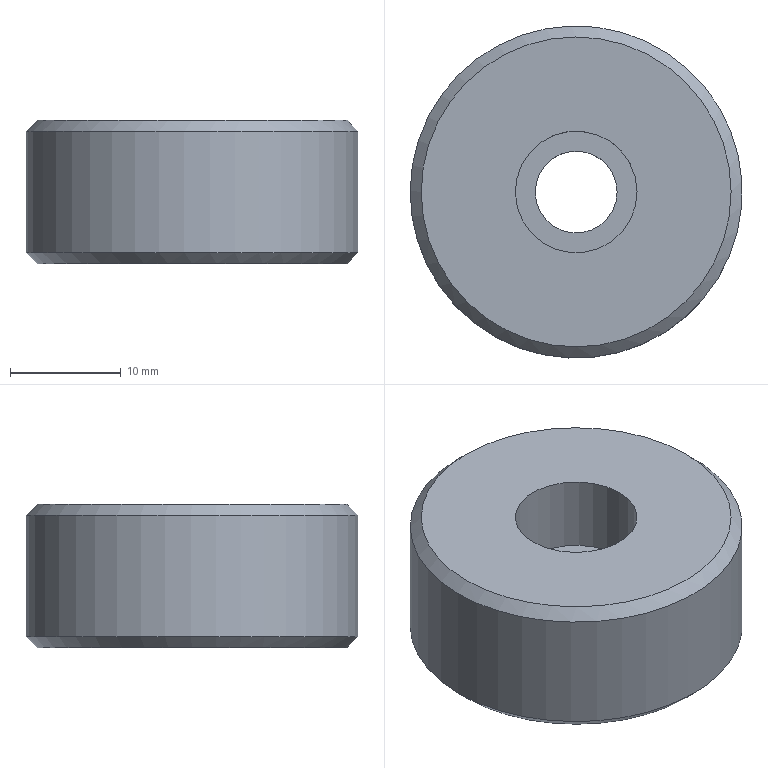Part | STEP file | solid 173 | 1 solid | 8 faces | box 30 x 30 x 13 mm | volume 8174 mm3 | plane 3 | cylinder 3 | cone 2 | commonest cylinder face diameters 7.4 x1 11 x1 30 x1